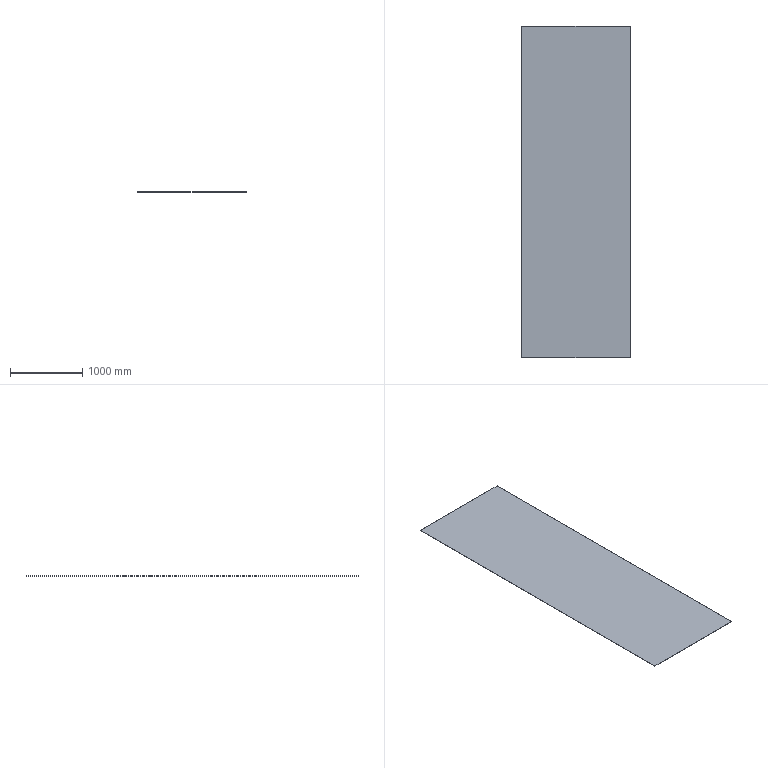Part | STEP file | 电柜通道花纹Plate 1 | 1 solid | 6 faces | box 1500 x 4585 x 4 mm | volume 27510000 mm3 | plane 6
STEP:
#1=CARTESIAN_POINT('',(0.,0.,0.));
#2=DIRECTION('',(0.,0.,1.));
#3=DIRECTION('',(1.,0.,0.));
#4=AXIS2_PLACEMENT_3D('',#1,#2,#3);
#5=CARTESIAN_POINT('',(1048.964,3141.263,0.));
#6=VERTEX_POINT('',#5);
#7=CARTESIAN_POINT('',(1048.964,-1443.737,0.));
#8=VERTEX_POINT('',#7);
#9=CARTESIAN_POINT('',(1048.964,0.,0.));
#10=DIRECTION('',(0.,-1.,0.));
#11=VECTOR('',#10,1.);
#12=LINE('',#9,#11);
#13=CARTESIAN_POINT('',(1048.964,0.,4.));
#14=DIRECTION('',(1.,0.,0.));
#15=DIRECTION('',(0.,0.,-1.));
#16=AXIS2_PLACEMENT_3D('',#13,#14,#15);
#17=PLANE('',#16);
#18=CARTESIAN_POINT('',(4.,0.));
#19=DIRECTION('',(0.,-1.));
#20=VECTOR('',#19,1.);
#21=LINE('',#18,#20);
#22=(GEOMETRIC_REPRESENTATION_CONTEXT(2)PARAMETRIC_REPRESENTATION_CONTEXT()REPRESENTATION_CONTEXT('',''));
#23=DEFINITIONAL_REPRESENTATION('',(#21),#22);
#24=PCURVE('',#17,#23);
#25=CARTESIAN_POINT('',(0.,0.,0.));
#26=DIRECTION('',(0.,0.,1.));
#27=DIRECTION('',(1.,0.,0.));
#28=AXIS2_PLACEMENT_3D('',#25,#26,#27);
#29=PLANE('',#28);
#30=CARTESIAN_POINT('',(1048.964,0.));
#31=DIRECTION('',(0.,-1.));
#32=VECTOR('',#31,1.);
#33=LINE('',#30,#32);
#34=(GEOMETRIC_REPRESENTATION_CONTEXT(2)PARAMETRIC_REPRESENTATION_CONTEXT()REPRESENTATION_CONTEXT('',''));
#35=DEFINITIONAL_REPRESENTATION('',(#33),#34);
#36=PCURVE('',#29,#35);
#37=SURFACE_CURVE('',#12,(#24,#36),.PCURVE_S1.);
#38=EDGE_CURVE('',#6,#8,#37,.T.);
#39=ORIENTED_EDGE('',*,*,#38,.F.);
#40=CARTESIAN_POINT('',(1048.964,3141.263,4.));
#41=VERTEX_POINT('',#40);
#42=CARTESIAN_POINT('',(1048.964,3141.263,4.));
#43=DIRECTION('',(0.,0.,-1.));
#44=VECTOR('',#43,1.);
#45=LINE('',#42,#44);
#46=CARTESIAN_POINT('',(0.,3141.263));
#47=DIRECTION('',(1.,0.));
#48=VECTOR('',#47,1.);
#49=LINE('',#46,#48);
#50=(GEOMETRIC_REPRESENTATION_CONTEXT(2)PARAMETRIC_REPRESENTATION_CONTEXT()REPRESENTATION_CONTEXT('',''));
#51=DEFINITIONAL_REPRESENTATION('',(#49),#50);
#52=PCURVE('',#17,#51);
#53=CARTESIAN_POINT('',(0.,3141.263,4.));
#54=DIRECTION('',(0.,1.,0.));
#55=DIRECTION('',(-1.,0.,0.));
#56=AXIS2_PLACEMENT_3D('',#53,#54,#55);
#57=PLANE('',#56);
#58=CARTESIAN_POINT('',(-1048.964,0.));
#59=DIRECTION('',(0.,-1.));
#60=VECTOR('',#59,1.);
#61=LINE('',#58,#60);
#62=(GEOMETRIC_REPRESENTATION_CONTEXT(2)PARAMETRIC_REPRESENTATION_CONTEXT()REPRESENTATION_CONTEXT('',''));
#63=DEFINITIONAL_REPRESENTATION('',(#61),#62);
#64=PCURVE('',#57,#63);
#65=SURFACE_CURVE('',#45,(#52,#64),.PCURVE_S1.);
#66=EDGE_CURVE('',#41,#6,#65,.T.);
#67=ORIENTED_EDGE('',*,*,#66,.F.);
#68=CARTESIAN_POINT('',(1048.964,-1443.737,4.));
#69=VERTEX_POINT('',#68);
#70=CARTESIAN_POINT('',(1048.964,0.,4.));
#71=DIRECTION('',(0.,-1.,0.));
#72=VECTOR('',#71,1.);
#73=LINE('',#70,#72);
#74=CARTESIAN_POINT('',(0.,0.));
#75=DIRECTION('',(0.,-1.));
#76=VECTOR('',#75,1.);
#77=LINE('',#74,#76);
#78=(GEOMETRIC_REPRESENTATION_CONTEXT(2)PARAMETRIC_REPRESENTATION_CONTEXT()REPRESENTATION_CONTEXT('',''));
#79=DEFINITIONAL_REPRESENTATION('',(#77),#78);
#80=PCURVE('',#17,#79);
#81=CARTESIAN_POINT('',(0.,0.,4.));
#82=DIRECTION('',(0.,0.,1.));
#83=DIRECTION('',(1.,0.,0.));
#84=AXIS2_PLACEMENT_3D('',#81,#82,#83);
#85=PLANE('',#84);
#86=CARTESIAN_POINT('',(1048.964,0.));
#87=DIRECTION('',(0.,-1.));
#88=VECTOR('',#87,1.);
#89=LINE('',#86,#88);
#90=(GEOMETRIC_REPRESENTATION_CONTEXT(2)PARAMETRIC_REPRESENTATION_CONTEXT()REPRESENTATION_CONTEXT('',''));
#91=DEFINITIONAL_REPRESENTATION('',(#89),#90);
#92=PCURVE('',#85,#91);
#93=SURFACE_CURVE('',#73,(#80,#92),.PCURVE_S1.);
#94=EDGE_CURVE('',#41,#69,#93,.T.);
#95=ORIENTED_EDGE('',*,*,#94,.T.);
#96=CARTESIAN_POINT('',(1048.964,-1443.737,4.));
#97=DIRECTION('',(0.,0.,-1.));
#98=VECTOR('',#97,1.);
#99=LINE('',#96,#98);
#100=CARTESIAN_POINT('',(0.,-1443.737));
#101=DIRECTION('',(1.,0.));
#102=VECTOR('',#101,1.);
#103=LINE('',#100,#102);
#104=(GEOMETRIC_REPRESENTATION_CONTEXT(2)PARAMETRIC_REPRESENTATION_CONTEXT()REPRESENTATION_CONTEXT('',''));
#105=DEFINITIONAL_REPRESENTATION('',(#103),#104);
#106=PCURVE('',#17,#105);
#107=CARTESIAN_POINT('',(0.,-1443.737,4.));
#108=DIRECTION('',(0.,1.,0.));
#109=DIRECTION('',(0.,0.,1.));
#110=AXIS2_PLACEMENT_3D('',#107,#108,#109);
#111=PLANE('',#110);
#112=CARTESIAN_POINT('',(0.,1048.964));
#113=DIRECTION('',(-1.,0.));
#114=VECTOR('',#113,1.);
#115=LINE('',#112,#114);
#116=(GEOMETRIC_REPRESENTATION_CONTEXT(2)PARAMETRIC_REPRESENTATION_CONTEXT()REPRESENTATION_CONTEXT('',''));
#117=DEFINITIONAL_REPRESENTATION('',(#115),#116);
#118=PCURVE('',#111,#117);
#119=SURFACE_CURVE('',#99,(#106,#118),.PCURVE_S1.);
#120=EDGE_CURVE('',#69,#8,#119,.T.);
#121=ORIENTED_EDGE('',*,*,#120,.T.);
#122=EDGE_LOOP('',(#39,#67,#95,#121));
#123=FACE_BOUND('',#122,.T.);
#124=ADVANCED_FACE('',(#123),#17,.T.);
#125=CARTESIAN_POINT('',(-451.036,3141.263,0.));
#126=VERTEX_POINT('',#125);
#127=CARTESIAN_POINT('',(0.,3141.263,0.));
#128=DIRECTION('',(1.,0.,0.));
#129=VECTOR('',#128,1.);
#130=LINE('',#127,#129);
#131=CARTESIAN_POINT('',(0.,-4.));
#132=DIRECTION('',(-1.,0.));
#133=VECTOR('',#132,1.);
#134=LINE('',#131,#133);
#135=(GEOMETRIC_REPRESENTATION_CONTEXT(2)PARAMETRIC_REPRESENTATION_CONTEXT()REPRESENTATION_CONTEXT('',''));
#136=DEFINITIONAL_REPRESENTATION('',(#134),#135);
#137=PCURVE('',#57,#136);
#138=CARTESIAN_POINT('',(0.,3141.263));
#139=DIRECTION('',(1.,0.));
#140=VECTOR('',#139,1.);
#141=LINE('',#138,#140);
#142=(GEOMETRIC_REPRESENTATION_CONTEXT(2)PARAMETRIC_REPRESENTATION_CONTEXT()REPRESENTATION_CONTEXT('',''));
#143=DEFINITIONAL_REPRESENTATION('',(#141),#142);
#144=PCURVE('',#29,#143);
#145=SURFACE_CURVE('',#130,(#137,#144),.PCURVE_S1.);
#146=EDGE_CURVE('',#126,#6,#145,.T.);
#147=ORIENTED_EDGE('',*,*,#146,.F.);
#148=CARTESIAN_POINT('',(-451.036,3141.263,4.));
#149=VERTEX_POINT('',#148);
#150=CARTESIAN_POINT('',(-451.036,3141.263,4.));
#151=DIRECTION('',(0.,0.,-1.));
#152=VECTOR('',#151,1.);
#153=LINE('',#150,#152);
#154=CARTESIAN_POINT('',(451.036,0.));
#155=DIRECTION('',(0.,-1.));
#156=VECTOR('',#155,1.);
#157=LINE('',#154,#156);
#158=(GEOMETRIC_REPRESENTATION_CONTEXT(2)PARAMETRIC_REPRESENTATION_CONTEXT()REPRESENTATION_CONTEXT('',''));
#159=DEFINITIONAL_REPRESENTATION('',(#157),#158);
#160=PCURVE('',#57,#159);
#161=CARTESIAN_POINT('',(-451.036,0.,4.));
#162=DIRECTION('',(1.,0.,0.));
#163=DIRECTION('',(0.,0.,-1.));
#164=AXIS2_PLACEMENT_3D('',#161,#162,#163);
#165=PLANE('',#164);
#166=CARTESIAN_POINT('',(0.,3141.263));
#167=DIRECTION('',(1.,0.));
#168=VECTOR('',#167,1.);
#169=LINE('',#166,#168);
#170=(GEOMETRIC_REPRESENTATION_CONTEXT(2)PARAMETRIC_REPRESENTATION_CONTEXT()REPRESENTATION_CONTEXT('',''));
#171=DEFINITIONAL_REPRESENTATION('',(#169),#170);
#172=PCURVE('',#165,#171);
#173=SURFACE_CURVE('',#153,(#160,#172),.PCURVE_S1.);
#174=EDGE_CURVE('',#149,#126,#173,.T.);
#175=ORIENTED_EDGE('',*,*,#174,.F.);
#176=CARTESIAN_POINT('',(0.,3141.263,4.));
#177=DIRECTION('',(1.,0.,0.));
#178=VECTOR('',#177,1.);
#179=LINE('',#176,#178);
#180=CARTESIAN_POINT('',(0.,0.));
#181=DIRECTION('',(-1.,0.));
#182=VECTOR('',#181,1.);
#183=LINE('',#180,#182);
#184=(GEOMETRIC_REPRESENTATION_CONTEXT(2)PARAMETRIC_REPRESENTATION_CONTEXT()REPRESENTATION_CONTEXT('',''));
#185=DEFINITIONAL_REPRESENTATION('',(#183),#184);
#186=PCURVE('',#57,#185);
#187=CARTESIAN_POINT('',(0.,3141.263));
#188=DIRECTION('',(1.,0.));
#189=VECTOR('',#188,1.);
#190=LINE('',#187,#189);
#191=(GEOMETRIC_REPRESENTATION_CONTEXT(2)PARAMETRIC_REPRESENTATION_CONTEXT()REPRESENTATION_CONTEXT('',''));
#192=DEFINITIONAL_REPRESENTATION('',(#190),#191);
#193=PCURVE('',#85,#192);
#194=SURFACE_CURVE('',#179,(#186,#193),.PCURVE_S1.);
#195=EDGE_CURVE('',#149,#41,#194,.T.);
#196=ORIENTED_EDGE('',*,*,#195,.T.);
#197=ORIENTED_EDGE('',*,*,#66,.T.);
#198=EDGE_LOOP('',(#147,#175,#196,#197));
#199=FACE_BOUND('',#198,.T.);
#200=ADVANCED_FACE('',(#199),#57,.T.);
#201=CARTESIAN_POINT('',(-451.036,-1443.737,0.));
#202=VERTEX_POINT('',#201);
#203=CARTESIAN_POINT('',(-451.036,0.,0.));
#204=DIRECTION('',(0.,-1.,0.));
#205=VECTOR('',#204,1.);
#206=LINE('',#203,#205);
#207=CARTESIAN_POINT('',(4.,0.));
#208=DIRECTION('',(0.,-1.));
#209=VECTOR('',#208,1.);
#210=LINE('',#207,#209);
#211=(GEOMETRIC_REPRESENTATION_CONTEXT(2)PARAMETRIC_REPRESENTATION_CONTEXT()REPRESENTATION_CONTEXT('',''));
#212=DEFINITIONAL_REPRESENTATION('',(#210),#211);
#213=PCURVE('',#165,#212);
#214=CARTESIAN_POINT('',(-451.036,0.));
#215=DIRECTION('',(0.,-1.));
#216=VECTOR('',#215,1.);
#217=LINE('',#214,#216);
#218=(GEOMETRIC_REPRESENTATION_CONTEXT(2)PARAMETRIC_REPRESENTATION_CONTEXT()REPRESENTATION_CONTEXT('',''));
#219=DEFINITIONAL_REPRESENTATION('',(#217),#218);
#220=PCURVE('',#29,#219);
#221=SURFACE_CURVE('',#206,(#213,#220),.PCURVE_S1.);
#222=EDGE_CURVE('',#126,#202,#221,.T.);
#223=ORIENTED_EDGE('',*,*,#222,.T.);
#224=CARTESIAN_POINT('',(-451.036,-1443.737,4.));
#225=VERTEX_POINT('',#224);
#226=CARTESIAN_POINT('',(-451.036,-1443.737,4.));
#227=DIRECTION('',(0.,0.,-1.));
#228=VECTOR('',#227,1.);
#229=LINE('',#226,#228);
#230=CARTESIAN_POINT('',(0.,-1443.737));
#231=DIRECTION('',(1.,0.));
#232=VECTOR('',#231,1.);
#233=LINE('',#230,#232);
#234=(GEOMETRIC_REPRESENTATION_CONTEXT(2)PARAMETRIC_REPRESENTATION_CONTEXT()REPRESENTATION_CONTEXT('',''));
#235=DEFINITIONAL_REPRESENTATION('',(#233),#234);
#236=PCURVE('',#165,#235);
#237=CARTESIAN_POINT('',(0.,-451.036));
#238=DIRECTION('',(-1.,0.));
#239=VECTOR('',#238,1.);
#240=LINE('',#237,#239);
#241=(GEOMETRIC_REPRESENTATION_CONTEXT(2)PARAMETRIC_REPRESENTATION_CONTEXT()REPRESENTATION_CONTEXT('',''));
#242=DEFINITIONAL_REPRESENTATION('',(#240),#241);
#243=PCURVE('',#111,#242);
#244=SURFACE_CURVE('',#229,(#236,#243),.PCURVE_S1.);
#245=EDGE_CURVE('',#225,#202,#244,.T.);
#246=ORIENTED_EDGE('',*,*,#245,.F.);
#247=CARTESIAN_POINT('',(-451.036,0.,4.));
#248=DIRECTION('',(0.,-1.,0.));
#249=VECTOR('',#248,1.);
#250=LINE('',#247,#249);
#251=CARTESIAN_POINT('',(0.,0.));
#252=DIRECTION('',(0.,-1.));
#253=VECTOR('',#252,1.);
#254=LINE('',#251,#253);
#255=(GEOMETRIC_REPRESENTATION_CONTEXT(2)PARAMETRIC_REPRESENTATION_CONTEXT()REPRESENTATION_CONTEXT('',''));
#256=DEFINITIONAL_REPRESENTATION('',(#254),#255);
#257=PCURVE('',#165,#256);
#258=CARTESIAN_POINT('',(-451.036,0.));
#259=DIRECTION('',(0.,-1.));
#260=VECTOR('',#259,1.);
#261=LINE('',#258,#260);
#262=(GEOMETRIC_REPRESENTATION_CONTEXT(2)PARAMETRIC_REPRESENTATION_CONTEXT()REPRESENTATION_CONTEXT('',''));
#263=DEFINITIONAL_REPRESENTATION('',(#261),#262);
#264=PCURVE('',#85,#263);
#265=SURFACE_CURVE('',#250,(#257,#264),.PCURVE_S1.);
#266=EDGE_CURVE('',#149,#225,#265,.T.);
#267=ORIENTED_EDGE('',*,*,#266,.F.);
#268=ORIENTED_EDGE('',*,*,#174,.T.);
#269=EDGE_LOOP('',(#223,#246,#267,#268));
#270=FACE_BOUND('',#269,.T.);
#271=ADVANCED_FACE('',(#270),#165,.F.);
#272=CARTESIAN_POINT('',(0.,-1443.737,0.));
#273=DIRECTION('',(1.,0.,0.));
#274=VECTOR('',#273,1.);
#275=LINE('',#272,#274);
#276=CARTESIAN_POINT('',(-4.,0.));
#277=DIRECTION('',(0.,1.));
#278=VECTOR('',#277,1.);
#279=LINE('',#276,#278);
#280=(GEOMETRIC_REPRESENTATION_CONTEXT(2)PARAMETRIC_REPRESENTATION_CONTEXT()REPRESENTATION_CONTEXT('',''));
#281=DEFINITIONAL_REPRESENTATION('',(#279),#280);
#282=PCURVE('',#111,#281);
#283=CARTESIAN_POINT('',(0.,-1443.737));
#284=DIRECTION('',(1.,0.));
#285=VECTOR('',#284,1.);
#286=LINE('',#283,#285);
#287=(GEOMETRIC_REPRESENTATION_CONTEXT(2)PARAMETRIC_REPRESENTATION_CONTEXT()REPRESENTATION_CONTEXT('',''));
#288=DEFINITIONAL_REPRESENTATION('',(#286),#287);
#289=PCURVE('',#29,#288);
#290=SURFACE_CURVE('',#275,(#282,#289),.PCURVE_S1.);
#291=EDGE_CURVE('',#202,#8,#290,.T.);
#292=ORIENTED_EDGE('',*,*,#291,.T.);
#293=ORIENTED_EDGE('',*,*,#120,.F.);
#294=CARTESIAN_POINT('',(0.,-1443.737,4.));
#295=DIRECTION('',(1.,0.,0.));
#296=VECTOR('',#295,1.);
#297=LINE('',#294,#296);
#298=CARTESIAN_POINT('',(0.,0.));
#299=DIRECTION('',(0.,1.));
#300=VECTOR('',#299,1.);
#301=LINE('',#298,#300);
#302=(GEOMETRIC_REPRESENTATION_CONTEXT(2)PARAMETRIC_REPRESENTATION_CONTEXT()REPRESENTATION_CONTEXT('',''));
#303=DEFINITIONAL_REPRESENTATION('',(#301),#302);
#304=PCURVE('',#111,#303);
#305=CARTESIAN_POINT('',(0.,-1443.737));
#306=DIRECTION('',(1.,0.));
#307=VECTOR('',#306,1.);
#308=LINE('',#305,#307);
#309=(GEOMETRIC_REPRESENTATION_CONTEXT(2)PARAMETRIC_REPRESENTATION_CONTEXT()REPRESENTATION_CONTEXT('',''));
#310=DEFINITIONAL_REPRESENTATION('',(#308),#309);
#311=PCURVE('',#85,#310);
#312=SURFACE_CURVE('',#297,(#304,#311),.PCURVE_S1.);
#313=EDGE_CURVE('',#225,#69,#312,.T.);
#314=ORIENTED_EDGE('',*,*,#313,.F.);
#315=ORIENTED_EDGE('',*,*,#245,.T.);
#316=EDGE_LOOP('',(#292,#293,#314,#315));
#317=FACE_BOUND('',#316,.T.);
#318=ADVANCED_FACE('',(#317),#111,.F.);
#319=ORIENTED_EDGE('',*,*,#94,.F.);
#320=ORIENTED_EDGE('',*,*,#195,.F.);
#321=ORIENTED_EDGE('',*,*,#266,.T.);
#322=ORIENTED_EDGE('',*,*,#313,.T.);
#323=EDGE_LOOP('',(#319,#320,#321,#322));
#324=FACE_BOUND('',#323,.T.);
#325=ADVANCED_FACE('',(#324),#85,.T.);
#326=ORIENTED_EDGE('',*,*,#38,.T.);
#327=ORIENTED_EDGE('',*,*,#291,.F.);
#328=ORIENTED_EDGE('',*,*,#222,.F.);
#329=ORIENTED_EDGE('',*,*,#146,.T.);
#330=EDGE_LOOP('',(#326,#327,#328,#329));
#331=FACE_BOUND('',#330,.T.);
#332=ADVANCED_FACE('',(#331),#29,.F.);
#333=CLOSED_SHELL('',(#124,#200,#271,#318,#325,#332));
#334=MANIFOLD_SOLID_BREP('',#333);
#335=(LENGTH_UNIT()NAMED_UNIT(*)SI_UNIT(.MILLI.,.METRE.));
#336=UNCERTAINTY_MEASURE_WITH_UNIT(LENGTH_MEASURE(0.0000001),#335,'','');
#337=(NAMED_UNIT(*)PLANE_ANGLE_UNIT()SI_UNIT($,.RADIAN.));
#338=(NAMED_UNIT(*)SI_UNIT($,.STERADIAN.)SOLID_ANGLE_UNIT());
#339=(GEOMETRIC_REPRESENTATION_CONTEXT(3)GLOBAL_UNCERTAINTY_ASSIGNED_CONTEXT((#336))GLOBAL_UNIT_ASSIGNED_CONTEXT((#335,#337,#338))REPRESENTATION_CONTEXT('',''));
#340=ADVANCED_BREP_SHAPE_REPRESENTATION('',(#4,#334),#339);